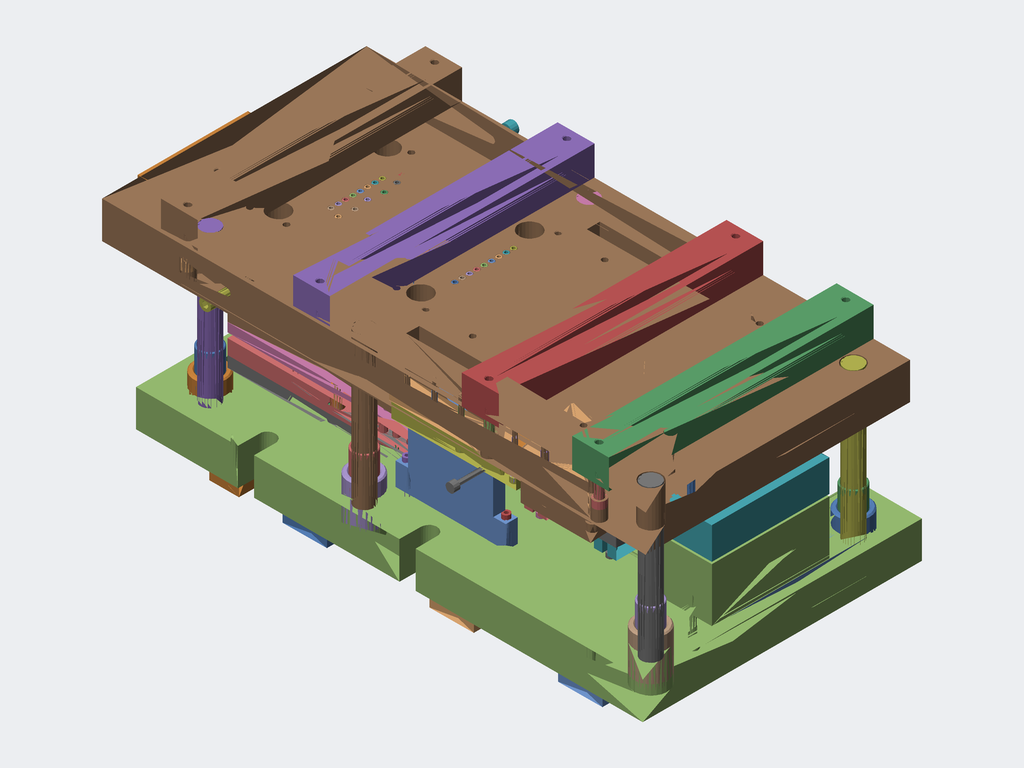Assembly | STEP file | 613 different items | 613 placed
Parts list (item | quantity | size | volume):
1 | x1 | 60 x 360 x 20 mm | 425296 mm3
2 | x1 | 40 x 360 x 20 mm | 281296 mm3
3 | x1 | 50 x 360 x 40 mm | 715429 mm3
4 | x1 | 50 x 360 x 40 mm | 715429 mm3
5 | x1 | 50 x 360 x 40 mm | 715429 mm3
6 | x1 | 50 x 360 x 40 mm | 715429 mm3
7 | x1 | 12 x 108 x 12 mm | 3732 mm3
8 | x1 | 12 x 108 x 12 mm | 3732 mm3
9 | x1 | 25 x 25 x 37 mm | 14578 mm3
10 | x1 | 6 x 42.771 x 14.853 mm | 2506 mm3
11 | x1 | 8 x 8 x 30 mm | 1498 mm3
12 | x1 | 8 x 8 x 30 mm | 1498 mm3
13 | x1 | 6 x 6 x 25 mm | 699.37 mm3
14 | x1 | 8 x 8 x 40 mm | 2000 mm3
15 | x1 | 8 x 8 x 40 mm | 2000 mm3
16 | x1 | 25 x 5 x 5 mm | 484.734 mm3
17 | x1 | 25 x 25 x 37 mm | 14578 mm3
18 | x1 | 24.97 x 5.97 x 55 mm | 8152 mm3
19 | x1 | 8 x 8 x 55 mm | 2684 mm3
20 | x1 | 8 x 8 x 30 mm | 1427 mm3
21 | x1 | 20 x 20 x 5 mm | 1265 mm3
22 | x1 | 6 x 6 x 36.5 mm | 342.826 mm3
23 | x1 | 6 x 6 x 36.5 mm | 342.826 mm3
24 | x1 | 6 x 6 x 36.5 mm | 342.826 mm3
25 | x1 | 6 x 6 x 36.5 mm | 342.826 mm3
26 | x1 | 6 x 6 x 36.5 mm | 342.826 mm3
27 | x1 | 6 x 6 x 36.5 mm | 342.826 mm3
28 | x1 | 6 x 6 x 36.5 mm | 342.826 mm3
29 | x1 | 6 x 6 x 36.5 mm | 342.826 mm3
30 | x1 | 6 x 6 x 36.5 mm | 342.826 mm3
31 | x1 | 6 x 6 x 36.5 mm | 342.826 mm3
32 | x1 | 6 x 6 x 36.5 mm | 342.826 mm3
33 | x1 | 6 x 6 x 36.5 mm | 342.826 mm3
34 | x1 | 6 x 6 x 36.5 mm | 342.826 mm3
35 | x1 | 6 x 6 x 36.5 mm | 342.826 mm3
36 | x1 | 6 x 6 x 36.5 mm | 342.826 mm3
37 | x1 | 6 x 6 x 36.5 mm | 342.826 mm3
38 | x1 | 6 x 6 x 36.5 mm | 342.826 mm3
39 | x1 | 6 x 6 x 36.5 mm | 342.826 mm3
40 | x1 | 6 x 6 x 36.5 mm | 342.826 mm3
41 | x1 | 6 x 6 x 36.5 mm | 342.826 mm3
42 | x1 | 6 x 6 x 36.5 mm | 342.826 mm3
43 | x1 | 6 x 6 x 36.5 mm | 342.826 mm3
44 | x1 | 6 x 6 x 36.5 mm | 342.826 mm3
45 | x1 | 6 x 6 x 36.5 mm | 342.826 mm3
46 | x1 | 5 x 5 x 25 mm | 484.734 mm3
47 | x1 | 12 x 12 x 4 mm | 331.627 mm3
48 | x1 | 12 x 12 x 4 mm | 331.627 mm3
49 | x1 | 12 x 12 x 4 mm | 331.627 mm3
50 | x1 | 12 x 12 x 4 mm | 331.627 mm3
51 | x1 | 12 x 12 x 4 mm | 331.627 mm3
52 | x1 | 12 x 12 x 4 mm | 331.627 mm3
53 | x1 | 8 x 8 x 50 mm | 2474 mm3
54 | x1 | 8 x 8 x 50 mm | 2474 mm3
55 | x1 | - | 125.363 mm3
56 | x1 | - | 125.363 mm3
57 | x1 | - | 125.363 mm3
58 | x1 | 29.97 x 5.97 x 55 mm | 9793 mm3
59 | x1 | 29.97 x 5.97 x 55 mm | 9793 mm3
60 | x1 | 24.97 x 9.97 x 55 mm | 13645 mm3
61 | x1 | 24.97 x 9.97 x 55 mm | 13645 mm3
62 | x1 | 25 x 130 x 15 mm | 47092 mm3
63 | x1 | 25 x 105.8 x 15 mm | 36908 mm3
64 | x1 | 25 x 16 x 80 mm | 27687 mm3
65 | x1 | 25 x 16 x 80 mm | 27687 mm3
66 | x1 | 150 x 150 x 43 mm | 782567 mm3
67 | x1 | 6 x 6 x 31.4 mm | 306.777 mm3
68 | x1 | 6 x 6 x 31.4 mm | 306.777 mm3
69 | x1 | 6 x 6 x 31.4 mm | 306.777 mm3
70 | x1 | 6 x 6 x 31.4 mm | 306.777 mm3
71 | x1 | 6 x 6 x 31.4 mm | 306.777 mm3
72 | x1 | 6 x 6 x 31.4 mm | 306.777 mm3
73 | x1 | 6 x 6 x 31.4 mm | 306.777 mm3
74 | x1 | 6 x 6 x 31.4 mm | 306.777 mm3
75 | x1 | 6 x 6 x 31.4 mm | 306.777 mm3
76 | x1 | 6 x 6 x 31.4 mm | 306.777 mm3
77 | x1 | 6 x 6 x 31.4 mm | 306.777 mm3
78 | x1 | 6 x 6 x 31.4 mm | 306.777 mm3
79 | x1 | 6 x 6 x 31.4 mm | 306.777 mm3
80 | x1 | 6 x 6 x 31.4 mm | 306.777 mm3
81 | x1 | 6 x 6 x 31.4 mm | 306.777 mm3
82 | x1 | 6 x 6 x 30.5 mm | 300.415 mm3
83 | x1 | 6 x 6 x 30.5 mm | 300.415 mm3
84 | x1 | 6 x 6 x 30.5 mm | 300.415 mm3
85 | x1 | 6 x 6 x 30.5 mm | 300.415 mm3
86 | x1 | 6 x 6 x 30.5 mm | 300.415 mm3
87 | x1 | 6 x 6 x 30.5 mm | 300.415 mm3
88 | x1 | 6 x 6 x 30.5 mm | 300.415 mm3
89 | x1 | 6 x 6 x 30.5 mm | 300.415 mm3
90 | x1 | 6 x 6 x 30.5 mm | 300.415 mm3
91 | x1 | 6 x 6 x 30.5 mm | 300.415 mm3
92 | x1 | 6 x 6 x 30.5 mm | 300.415 mm3
93 | x1 | 6 x 6 x 30.5 mm | 300.415 mm3
94 | x1 | 6 x 6 x 30.5 mm | 300.415 mm3
95 | x1 | 6 x 6 x 30.5 mm | 300.415 mm3
96 | x1 | 6 x 6 x 30.5 mm | 300.415 mm3
97 | x1 | 6 x 6 x 24.2 mm | 255.883 mm3
98 | x1 | 6 x 6 x 24.2 mm | 255.883 mm3
99 | x1 | 6 x 6 x 24.2 mm | 255.883 mm3
100 | x1 | 6 x 6 x 24.2 mm | 255.883 mm3
101 | x1 | 6 x 6 x 24.2 mm | 255.883 mm3
102 | x1 | 6 x 6 x 24.2 mm | 255.883 mm3
103 | x1 | 6 x 6 x 24.2 mm | 255.883 mm3
104 | x1 | 6 x 6 x 24.2 mm | 255.883 mm3
105 | x1 | 6 x 6 x 24.2 mm | 255.883 mm3
106 | x1 | 6 x 6 x 24.2 mm | 255.883 mm3
107 | x1 | 6 x 6 x 24.2 mm | 255.883 mm3
108 | x1 | 6 x 6 x 24.2 mm | 255.883 mm3
109 | x1 | 6 x 6 x 24.2 mm | 255.883 mm3
110 | x1 | 6 x 6 x 24.2 mm | 255.883 mm3
111 | x1 | 6 x 6 x 24.2 mm | 255.883 mm3
112 | x1 | 6 x 6 x 24.2 mm | 255.883 mm3
113 | x1 | 6 x 6 x 24.2 mm | 255.883 mm3
114 | x1 | 6 x 6 x 24.2 mm | 255.883 mm3
115 | x1 | 6 x 6 x 30.5 mm | 300.415 mm3
116 | x1 | 8 x 8 x 55 mm | 2726 mm3
117 | x1 | 8 x 8 x 55 mm | 2726 mm3
118 | x1 | 8 x 8 x 55 mm | 2726 mm3
119 | x1 | 8 x 8 x 55 mm | 2726 mm3
120 | x1 | 22 x 22 x 5 mm | 1608 mm3
121 | x1 | 170 x 20 x 20 mm | 54220 mm3
122 | x1 | 170 x 20 x 20 mm | 54220 mm3
123 | x1 | 275 x 320 x 12 mm | 986186 mm3
124 | x1 | 150 x 16 x 219.952 mm | 343529 mm3
125 | x1 | 114.24 x 2.3 x 30 mm | 5016 mm3
126 | x1 | 114.24 x 2.3 x 30 mm | 5016 mm3
127 | x1 | 114.24 x 2.3 x 30 mm | 5016 mm3
128 | x1 | 112 x 4.97 x 28.8 mm | 6489 mm3
129 | x1 | 112 x 4.97 x 28.8 mm | 6489 mm3
130 | x1 | 112 x 4.97 x 28.8 mm | 6489 mm3
131 | x1 | 110 x 5 x 24.6 mm | 7286 mm3
132 | x1 | 110 x 5 x 24.6 mm | 7286 mm3
133 | x1 | 110 x 5 x 24.6 mm | 7286 mm3
134 | x1 | 740 x 360 x 50 mm | 12464392 mm3
135 | x1 | 110 x 4.97 x 20 mm | 4432 mm3
136 | x1 | 110 x 4.97 x 20 mm | 4432 mm3
137 | x1 | 110 x 4.97 x 20 mm | 4432 mm3
138 | x1 | 110 x 4.97 x 20 mm | 4432 mm3
139 | x1 | 110 x 4.97 x 20 mm | 4432 mm3
140 | x1 | 114.24 x 2.3 x 30 mm | 5016 mm3
141 | x1 | 149 x 120 x 21.74 mm | 329380 mm3
142 | x1 | 28 x 28 x 35 mm | 8179 mm3
143 | x1 | 28 x 28 x 35 mm | 8179 mm3
144 | x1 | 28 x 28 x 35 mm | 8179 mm3
145 | x1 | 28 x 28 x 35 mm | 8179 mm3
146 | x1 | 28 x 28 x 35 mm | 8179 mm3
147 | x1 | 28 x 28 x 35 mm | 8179 mm3
148 | x1 | 28 x 28 x 35 mm | 8179 mm3
149 | x1 | 270 x 210 x 20 mm | 990769 mm3
150 | x1 | 270 x 210 x 20 mm | 665006 mm3
151 | x1 | 270 x 210 x 12 mm | 556019 mm3
152 | x1 | 270 x 210 x 15 mm | 687226 mm3
153 | x1 | 16 x 16 x 16 mm | 2762 mm3
154 | x1 | 22 x 17 x 50.8 mm | 13403 mm3
155 | x1 | 16 x 16 x 16 mm | 2762 mm3
156 | x1 | 22 x 100 x 29.5 mm | 60333 mm3
157 | x1 | 6 x 38.927 x 27.874 mm | 2506 mm3
158 | x1 | 30 x 210 x 15 mm | 89928 mm3
159 | x1 | 30 x 15 x 75 mm | 33035 mm3
160 | x1 | 22 x 17 x 50.8 mm | 13403 mm3
161 | x1 | 14 x 153 x 10 mm | 17764 mm3
162 | x1 | 60 x 288 x 31.2 mm | 374640 mm3
163 | x1 | 30 x 15 x 75 mm | 32986 mm3
164 | x1 | 27.92 x 20 x 22.9 mm | 8682 mm3
165 | x1 | 27.92 x 20 x 22.9 mm | 8682 mm3
166 | x1 | 95 x 320 x 31.2 mm | 758918 mm3
167 | x1 | 30 x 15 x 75 mm | 32980 mm3
168 | x1 | 30 x 15 x 75 mm | 33035 mm3
169 | x1 | 150 x 16 x 219.952 mm | 343529 mm3
170 | x1 | 30 x 210 x 15 mm | 89928 mm3
171 | x1 | 20 x 156 x 23.01 mm | 61919 mm3
172 | x1 | 22 x 17 x 50.8 mm | 13297 mm3
173 | x1 | 22 x 100 x 29.5 mm | 60684 mm3
174 | x1 | 14 x 153 x 10 mm | 17762 mm3
175 | x1 | 22 x 17 x 50.8 mm | 13297 mm3
176 | x1 | 110 x 5 x 24.6 mm | 7286 mm3
177 | x1 | 150 x 135 x 10 mm | 124052 mm3
178 | x1 | 118 x 5 x 53.54 mm | 21080 mm3
179 | x1 | 118 x 5 x 53.54 mm | 21081 mm3
180 | x1 | 118 x 5 x 53.54 mm | 21080 mm3
181 | x1 | 118 x 5 x 53.54 mm | 21081 mm3
182 | x1 | 118 x 5 x 53.54 mm | 21080 mm3
183 | x1 | 136 x 1.85 x 22 mm | 2666 mm3
184 | x1 | 136 x 1.85 x 22 mm | 2666 mm3
185 | x1 | 136 x 1.85 x 22 mm | 2666 mm3
186 | x1 | 136 x 1.85 x 22 mm | 2666 mm3
187 | x1 | 136 x 1.85 x 22 mm | 2666 mm3
188 | x1 | 136 x 1.85 x 22 mm | 2666 mm3
189 | x1 | 136 x 1.85 x 22 mm | 2666 mm3
190 | x1 | 136 x 1.85 x 22 mm | 2666 mm3
191 | x1 | 112 x 4.97 x 28.8 mm | 6489 mm3
192 | x1 | 28 x 28 x 35 mm | 8179 mm3
193 | x1 | 150 x 135 x 15 mm | 212258 mm3
194 | x1 | 39.94 x 2.4 x 27.2 mm | 2495 mm3
195 | x1 | 39.94 x 2.4 x 27.2 mm | 2495 mm3
196 | x1 | 39.94 x 2.4 x 27.2 mm | 2495 mm3
197 | x1 | 39.94 x 2.4 x 27.2 mm | 2495 mm3
198 | x1 | 39.94 x 2.4 x 27.2 mm | 2495 mm3
199 | x1 | 39.94 x 2.4 x 27.2 mm | 2495 mm3
200 | x1 | 39.94 x 2.4 x 27.2 mm | 2495 mm3
201 | x1 | 39.94 x 2.4 x 27.2 mm | 2495 mm3
202 | x1 | 39.94 x 2.4 x 27.2 mm | 2495 mm3
203 | x1 | 39.94 x 2.4 x 27.2 mm | 2495 mm3
204 | x1 | 39.94 x 2.4 x 27.2 mm | 2495 mm3
205 | x1 | 55 x 14 x 9.8 mm | 5918 mm3
206 | x1 | 60 x 14 x 9.8 mm | 6535 mm3
207 | x1 | 39.94 x 2.4 x 27.2 mm | 2495 mm3
208 | x1 | 39.94 x 2.4 x 27.2 mm | 2495 mm3
209 | x1 | 34.97 x 6 x 32.7 mm | 4654 mm3
210 | x1 | 34.97 x 6 x 32.7 mm | 4654 mm3
211 | x1 | 39.94 x 2.4 x 27.2 mm | 2495 mm3
212 | x1 | 39.94 x 2.4 x 27.2 mm | 2495 mm3
213 | x1 | 39.94 x 2.4 x 27.2 mm | 2495 mm3
214 | x1 | 39.94 x 2.4 x 27.2 mm | 2495 mm3
215 | x1 | 39.94 x 2.4 x 27.2 mm | 2495 mm3
216 | x1 | 22 x 22 x 5 mm | 1608 mm3
217 | x1 | 12 x 12 x 32 mm | 2552 mm3
218 | x1 | 12 x 12 x 32 mm | 2552 mm3
219 | x1 | 22 x 22 x 5 mm | 1608 mm3
220 | x1 | 22 x 22 x 5 mm | 1608 mm3
221 | x1 | 12 x 12 x 32 mm | 2552 mm3
222 | x1 | 22 x 22 x 5 mm | 1608 mm3
223 | x1 | 12 x 12 x 32 mm | 2552 mm3
224 | x1 | 22 x 22 x 5 mm | 1608 mm3
225 | x1 | 12 x 12 x 32 mm | 2552 mm3
226 | x1 | 16 x 16 x 27 mm | 3890 mm3
227 | x1 | 25 x 25 x 5 mm | 2168 mm3
228 | x1 | 16 x 16 x 27 mm | 3890 mm3
229 | x1 | 25 x 25 x 5 mm | 2168 mm3
230 | x1 | 16 x 16 x 27 mm | 3890 mm3
231 | x1 | 25 x 25 x 5 mm | 2168 mm3
232 | x1 | 25 x 25 x 5 mm | 2168 mm3
233 | x1 | 16 x 16 x 27 mm | 3890 mm3
234 | x1 | 16 x 16 x 27 mm | 3890 mm3
235 | x1 | 25 x 25 x 5 mm | 2168 mm3
236 | x1 | 16 x 16 x 27 mm | 3890 mm3
237 | x1 | 25 x 25 x 5 mm | 2168 mm3
238 | x1 | 16 x 16 x 27 mm | 3890 mm3
239 | x1 | 25 x 25 x 5 mm | 2168 mm3
240 | x1 | 14 x 14 x 27 mm | 2618 mm3
241 | x1 | 20 x 20 x 5 mm | 1265 mm3
242 | x1 | 14 x 14 x 27 mm | 2618 mm3
243 | x1 | 20 x 20 x 5 mm | 1265 mm3
244 | x1 | 14 x 14 x 27 mm | 2618 mm3
245 | x1 | 20 x 20 x 5 mm | 1265 mm3
246 | x1 | 14 x 14 x 27 mm | 2618 mm3
247 | x1 | 20 x 20 x 5 mm | 1265 mm3
248 | x1 | 14 x 14 x 27 mm | 2618 mm3
249 | x1 | 20 x 20 x 5 mm | 1265 mm3
250 | x1 | 25 x 25 x 5 mm | 2168 mm3
251 | x1 | 16 x 16 x 27 mm | 3890 mm3
252 | x1 | 14 x 14 x 27 mm | 2618 mm3
253 | x1 | 12 x 12 x 32 mm | 2552 mm3
254 | x1 | 270 x 210 x 20 mm | 936503 mm3
255 | x1 | 22 x 22 x 35 mm | 3894 mm3
256 | x1 | 22 x 22 x 35 mm | 3894 mm3
257 | x1 | 22 x 22 x 35 mm | 3894 mm3
258 | x1 | 22 x 22 x 35 mm | 3894 mm3
259 | x1 | 22 x 22 x 35 mm | 3894 mm3
260 | x1 | 22 x 22 x 35 mm | 3894 mm3
261 | x1 | 25 x 25 x 45 mm | 5947 mm3
262 | x1 | 25 x 25 x 45 mm | 5947 mm3
263 | x1 | 25 x 25 x 45 mm | 5947 mm3
264 | x1 | 25 x 25 x 45 mm | 5947 mm3
265 | x1 | 25 x 25 x 45 mm | 5947 mm3
266 | x1 | 25 x 25 x 45 mm | 5947 mm3
267 | x1 | 25 x 25 x 45 mm | 5947 mm3
268 | x1 | 25 x 25 x 45 mm | 5947 mm3
269 | x1 | 690 x 380 x 50 mm | 10135272 mm3
270 | x1 | 270 x 210 x 25 mm | 722658 mm3
271 | x1 | 12 x 12 x 46 mm | 1731 mm3
272 | x1 | 18 x 18 x 9.92 mm | 1371 mm3
273 | x1 | 20 x 156 x 23.01 mm | 61919 mm3
274 | x1 | 12 x 12 x 46 mm | 1731 mm3
275 | x1 | 18 x 18 x 9.92 mm | 1371 mm3
276 | x1 | 5.998 x 5.997 x 50.45 mm | 77.124 mm3
277 | x1 | 5.998 x 5.997 x 50.45 mm | 77.124 mm3
278 | x1 | 6 x 6 x 50 mm | 346.471 mm3
279 | x1 | 6 x 6 x 50 mm | 346.471 mm3
280 | x1 | 5.998 x 5.997 x 50.45 mm | 77.124 mm3
281 | x1 | 6 x 6 x 50 mm | 346.471 mm3
282 | x1 | 5.998 x 5.997 x 50.45 mm | 77.124 mm3
283 | x1 | 6 x 6 x 50 mm | 346.471 mm3
284 | x1 | 5.998 x 5.997 x 50.45 mm | 77.124 mm3
285 | x1 | 6 x 6 x 50 mm | 346.471 mm3
286 | x1 | 6 x 6 x 50 mm | 346.471 mm3
287 | x1 | 5.998 x 5.997 x 50.45 mm | 77.124 mm3
288 | x1 | 6 x 6 x 50 mm | 346.471 mm3
289 | x1 | 6 x 6 x 50 mm | 346.471 mm3
290 | x1 | 6 x 6 x 50 mm | 346.471 mm3
291 | x1 | 5.998 x 5.997 x 50.45 mm | 77.124 mm3
292 | x1 | 5.998 x 5.997 x 50.45 mm | 77.124 mm3
293 | x1 | 5.998 x 5.997 x 50.45 mm | 77.124 mm3
294 | x1 | 6 x 6 x 50 mm | 346.471 mm3
295 | x1 | 6 x 6 x 50 mm | 346.471 mm3
296 | x1 | 5.998 x 5.997 x 50.45 mm | 77.124 mm3
297 | x1 | 5.998 x 5.997 x 50.45 mm | 77.124 mm3
298 | x1 | 5.998 x 5.997 x 50.45 mm | 77.124 mm3
299 | x1 | 6 x 6 x 50 mm | 346.471 mm3
300 | x1 | 8 x 8 x 55 mm | 2684 mm3
301 | x1 | 8 x 8 x 55 mm | 2684 mm3
302 | x1 | 8 x 8 x 55 mm | 2684 mm3
303 | x1 | 8 x 8 x 30 mm | 1427 mm3
304 | x1 | 8 x 8 x 30 mm | 1427 mm3
305 | x1 | 8 x 8 x 30 mm | 1427 mm3
306 | x1 | 10 x 10 x 51 mm | 1658 mm3
307 | x1 | 10 x 10 x 51 mm | 1658 mm3
308 | x1 | 10 x 10 x 51 mm | 1658 mm3
309 | x1 | 10 x 10 x 51 mm | 1658 mm3
310 | x1 | 10 x 10 x 21 mm | 809.617 mm3
311 | x1 | 10 x 10 x 21 mm | 809.617 mm3
312 | x1 | 10 x 10 x 21 mm | 809.617 mm3
313 | x1 | 10 x 10 x 21 mm | 809.617 mm3
314 | x1 | 10 x 10 x 21 mm | 809.617 mm3
315 | x1 | 10 x 10 x 21 mm | 809.617 mm3
316 | x1 | 10 x 10 x 21 mm | 809.617 mm3
317 | x1 | 10 x 10 x 21 mm | 809.617 mm3
318 | x1 | 10 x 10 x 21 mm | 809.617 mm3
319 | x1 | 10 x 10 x 21 mm | 809.617 mm3
320 | x1 | 10 x 10 x 16 mm | 668.246 mm3
321 | x1 | 10 x 10 x 16 mm | 668.246 mm3
322 | x1 | 10 x 10 x 16 mm | 668.246 mm3
323 | x1 | 10 x 10 x 16 mm | 668.246 mm3
324 | x1 | 10 x 10 x 16 mm | 668.246 mm3
325 | x1 | 10 x 10 x 16 mm | 668.246 mm3
326 | x1 | 10 x 10 x 16 mm | 668.246 mm3
327 | x1 | 10 x 10 x 16 mm | 668.246 mm3
328 | x1 | 10 x 10 x 16 mm | 668.246 mm3
329 | x1 | 10 x 10 x 16 mm | 668.246 mm3
330 | x1 | 13 x 13 x 68 mm | 3913 mm3
331 | x1 | 13 x 13 x 68 mm | 3913 mm3
332 | x1 | 13 x 13 x 68 mm | 3913 mm3
333 | x1 | 13 x 13 x 68 mm | 3913 mm3
334 | x1 | 13 x 13 x 68 mm | 3913 mm3
335 | x1 | 13 x 13 x 68 mm | 3913 mm3
336 | x1 | 13 x 13 x 53 mm | 3159 mm3
337 | x1 | 13 x 13 x 53 mm | 3159 mm3
338 | x1 | 13 x 13 x 53 mm | 3159 mm3
339 | x1 | 13 x 13 x 53 mm | 3159 mm3
340 | x1 | 13 x 13 x 53 mm | 3159 mm3
341 | x1 | 13 x 13 x 53 mm | 3159 mm3
342 | x1 | 13 x 13 x 53 mm | 3159 mm3
343 | x1 | 13 x 13 x 53 mm | 3159 mm3
344 | x1 | 8 x 8 x 10 mm | 413.018 mm3
345 | x1 | 8 x 8 x 10 mm | 413.018 mm3
346 | x1 | 8 x 8 x 10 mm | 413.018 mm3
347 | x1 | 8 x 8 x 10 mm | 413.018 mm3
348 | x1 | 8 x 8 x 10 mm | 413.018 mm3
349 | x1 | 8 x 8 x 10 mm | 413.018 mm3
350 | x1 | 8 x 8 x 10 mm | 413.018 mm3
351 | x1 | 8 x 8 x 10 mm | 413.018 mm3
352 | x1 | 8 x 8 x 10 mm | 413.018 mm3
353 | x1 | 8 x 8 x 10 mm | 413.018 mm3
354 | x1 | 8 x 8 x 10 mm | 413.018 mm3
355 | x1 | 8 x 8 x 10 mm | 413.018 mm3
356 | x1 | 8 x 8 x 10 mm | 413.018 mm3
357 | x1 | 8 x 8 x 10 mm | 413.018 mm3
358 | x1 | 8 x 8 x 10 mm | 413.018 mm3
359 | x1 | 8 x 8 x 10 mm | 413.018 mm3
360 | x1 | 8 x 8 x 10 mm | 413.018 mm3
361 | x1 | 8 x 8 x 10 mm | 413.018 mm3
362 | x1 | 8 x 8 x 10 mm | 413.018 mm3
363 | x1 | 8 x 8 x 10 mm | 413.018 mm3
364 | x1 | 8 x 8 x 10 mm | 413.018 mm3
365 | x1 | 8 x 8 x 10 mm | 413.018 mm3
366 | x1 | 8 x 8 x 10 mm | 413.018 mm3
367 | x1 | 8 x 8 x 10 mm | 413.018 mm3
368 | x1 | 16 x 16 x 35 mm | 3608 mm3
369 | x1 | 16 x 16 x 35 mm | 3608 mm3
370 | x1 | 16 x 16 x 35 mm | 3608 mm3
371 | x1 | 16 x 16 x 35 mm | 3608 mm3
372 | x1 | 16 x 16 x 35 mm | 3608 mm3
373 | x1 | 16 x 16 x 35 mm | 3608 mm3
374 | x1 | 13 x 13 x 33 mm | 2154 mm3
375 | x1 | 13 x 13 x 33 mm | 2154 mm3
376 | x1 | 13 x 13 x 33 mm | 2154 mm3
377 | x1 | 13 x 13 x 33 mm | 2154 mm3
378 | x1 | 13 x 13 x 33 mm | 2154 mm3
379 | x1 | 13 x 13 x 33 mm | 2154 mm3
380 | x1 | 13 x 13 x 33 mm | 2154 mm3
381 | x1 | 13 x 13 x 33 mm | 2154 mm3
382 | x1 | 10 x 10 x 21 mm | 809.617 mm3
383 | x1 | 10 x 10 x 21 mm | 809.617 mm3
384 | x1 | 10 x 10 x 21 mm | 809.617 mm3
385 | x1 | 10 x 10 x 21 mm | 809.617 mm3
386 | x1 | 8.5 x 8.5 x 25 mm | 630.698 mm3
387 | x1 | 8.5 x 8.5 x 25 mm | 630.698 mm3
388 | x1 | 8.5 x 8.5 x 30 mm | 728.873 mm3
389 | x1 | 8.5 x 8.5 x 30 mm | 728.873 mm3
390 | x1 | 8.5 x 8.5 x 45 mm | 1023 mm3
391 | x1 | 8.5 x 8.5 x 45 mm | 1023 mm3
392 | x1 | 8.5 x 8.5 x 45 mm | 1023 mm3
393 | x1 | 16 x 50 x 16 mm | 4786 mm3
394 | x1 | 16 x 50 x 16 mm | 4786 mm3
395 | x1 | 16 x 16 x 50 mm | 4786 mm3
396 | x1 | 16 x 16 x 50 mm | 4786 mm3
397 | x1 | 16 x 16 x 50 mm | 4786 mm3
398 | x1 | 16 x 16 x 50 mm | 4786 mm3
399 | x1 | 16 x 16 x 50 mm | 4786 mm3
400 | x1 | 16 x 16 x 50 mm | 4786 mm3
401 | x1 | 16 x 16 x 50 mm | 4786 mm3
402 | x1 | 16 x 16 x 50 mm | 4786 mm3
403 | x1 | 13 x 13 x 58 mm | 3411 mm3
404 | x1 | 13 x 13 x 58 mm | 3411 mm3
405 | x1 | 13 x 13 x 58 mm | 3411 mm3
406 | x1 | 13 x 13 x 58 mm | 3411 mm3
407 | x1 | 13 x 13 x 58 mm | 3411 mm3
408 | x1 | 16 x 16 x 50 mm | 4786 mm3
409 | x1 | 16 x 16 x 50 mm | 4786 mm3
410 | x1 | 13 x 13 x 58 mm | 3411 mm3
411 | x1 | 10 x 10 x 21 mm | 809.617 mm3
412 | x1 | 10 x 10 x 21 mm | 809.617 mm3
413 | x1 | 10 x 10 x 21 mm | 809.617 mm3
414 | x1 | 10 x 10 x 21 mm | 809.617 mm3
415 | x1 | 10 x 10 x 21 mm | 809.617 mm3
416 | x1 | 10 x 10 x 21 mm | 809.617 mm3
417 | x1 | 13 x 13 x 48 mm | 2908 mm3
418 | x1 | 13 x 13 x 48 mm | 2908 mm3
419 | x1 | 5.5 x 5.5 x 48 mm | 378.644 mm3
420 | x1 | 5.5 x 5.5 x 48 mm | 378.644 mm3
421 | x1 | 5.5 x 5.5 x 48 mm | 378.644 mm3
422 | x1 | 5.5 x 5.5 x 48 mm | 378.644 mm3
423 | x1 | 5.5 x 5.5 x 48 mm | 378.644 mm3
424 | x1 | 5.5 x 5.5 x 48 mm | 378.644 mm3
425 | x1 | 5.5 x 5.5 x 48 mm | 378.644 mm3
426 | x1 | 5.5 x 5.5 x 48 mm | 378.644 mm3
427 | x1 | 8.5 x 8.5 x 25 mm | 577.553 mm3
428 | x1 | 8.5 x 8.5 x 25 mm | 577.553 mm3
429 | x1 | 8.5 x 8.5 x 25 mm | 577.553 mm3
430 | x1 | 8.5 x 8.5 x 25 mm | 577.553 mm3
431 | x1 | 10 x 10 x 21 mm | 809.617 mm3
432 | x1 | 10 x 10 x 21 mm | 809.617 mm3
433 | x1 | 10 x 10 x 21 mm | 809.617 mm3
434 | x1 | 10 x 10 x 21 mm | 809.617 mm3
435 | x1 | 10 x 10 x 21 mm | 809.617 mm3
436 | x1 | 10 x 10 x 21 mm | 809.617 mm3
437 | x1 | 10 x 10 x 21 mm | 809.617 mm3
438 | x1 | 10 x 10 x 21 mm | 809.617 mm3
439 | x1 | 10 x 10 x 36 mm | 1234 mm3
440 | x1 | 10 x 10 x 36 mm | 1234 mm3
441 | x1 | 10 x 10 x 36 mm | 1234 mm3
442 | x1 | 10 x 10 x 36 mm | 1234 mm3
443 | x1 | 10 x 10 x 51 mm | 1658 mm3
444 | x1 | 10 x 10 x 51 mm | 1658 mm3
445 | x1 | 10 x 10 x 51 mm | 1658 mm3
446 | x1 | 10 x 10 x 51 mm | 1658 mm3
447 | x1 | 10 x 10 x 51 mm | 1658 mm3
448 | x1 | 10 x 10 x 51 mm | 1658 mm3
449 | x1 | 10 x 10 x 51 mm | 1658 mm3
450 | x1 | 10 x 10 x 51 mm | 1658 mm3
451 | x1 | 10 x 10 x 51 mm | 1658 mm3
452 | x1 | 10 x 10 x 51 mm | 1658 mm3
453 | x1 | 13 x 13 x 58 mm | 3411 mm3
454 | x1 | 13 x 13 x 58 mm | 3411 mm3
455 | x1 | 13 x 13 x 58 mm | 3411 mm3
456 | x1 | 13 x 13 x 58 mm | 3411 mm3
457 | x1 | - | 70.891 mm3
458 | x1 | - | 70.891 mm3
459 | x1 | - | 70.891 mm3
460 | x1 | - | 70.891 mm3
461 | x1 | - | 70.891 mm3
462 | x1 | - | 70.891 mm3
463 | x1 | - | 70.891 mm3
464 | x1 | - | 70.891 mm3
465 | x1 | - | 70.891 mm3
466 | x1 | - | 70.891 mm3
467 | x1 | - | 70.891 mm3
468 | x1 | - | 70.891 mm3
469 | x1 | - | 70.891 mm3
470 | x1 | - | 70.891 mm3
471 | x1 | - | 70.891 mm3
472 | x1 | - | 70.891 mm3
473 | x1 | - | 70.891 mm3
474 | x1 | - | 70.891 mm3
475 | x1 | - | 70.891 mm3
476 | x1 | - | 70.891 mm3
477 | x1 | - | 70.891 mm3
478 | x1 | - | 70.891 mm3
479 | x1 | - | 70.891 mm3
480 | x1 | - | 70.891 mm3
481 | x1 | - | 70.891 mm3
482 | x1 | - | 70.891 mm3
483 | x1 | - | 70.891 mm3
484 | x1 | - | 70.891 mm3
485 | x1 | - | 70.891 mm3
486 | x1 | - | 70.891 mm3
487 | x1 | - | 70.891 mm3
488 | x1 | - | 70.891 mm3
489 | x1 | - | 70.891 mm3
490 | x1 | 6 x 6 x 40 mm | 281.648 mm3
491 | x1 | 6 x 6 x 40 mm | 281.648 mm3
492 | x1 | 6 x 6 x 40 mm | 281.648 mm3
493 | x1 | 6 x 6 x 40 mm | 281.648 mm3
494 | x1 | 6 x 6 x 40 mm | 281.648 mm3
495 | x1 | 6 x 6 x 40 mm | 281.648 mm3
496 | x1 | 6 x 6 x 40 mm | 281.648 mm3
497 | x1 | 6 x 6 x 40 mm | 281.648 mm3
498 | x1 | 6 x 6 x 40 mm | 281.648 mm3
499 | x1 | 6 x 6 x 40 mm | 281.648 mm3
500 | x1 | 6 x 6 x 40 mm | 281.648 mm3
501 | x1 | 6 x 6 x 40 mm | 281.648 mm3
502 | x1 | 6 x 6 x 40 mm | 281.648 mm3
503 | x1 | 6 x 6 x 40 mm | 281.648 mm3
504 | x1 | - | 70.891 mm3
505 | x1 | 6 x 6 x 40 mm | 281.648 mm3
506 | x1 | 8 x 8 x 10 mm | 413.018 mm3
507 | x1 | 8 x 8 x 10 mm | 413.018 mm3
508 | x1 | 8 x 8 x 10 mm | 413.018 mm3
509 | x1 | 8 x 8 x 10 mm | 413.018 mm3
510 | x1 | 8 x 8 x 10 mm | 413.018 mm3
511 | x1 | 8 x 8 x 10 mm | 413.018 mm3
512 | x1 | 8 x 8 x 10 mm | 413.018 mm3
513 | x1 | 8 x 8 x 10 mm | 413.018 mm3
514 | x1 | 8 x 8 x 10 mm | 413.018 mm3
515 | x1 | 8 x 8 x 10 mm | 413.018 mm3
516 | x1 | 8 x 8 x 10 mm | 413.018 mm3
517 | x1 | 8 x 8 x 10 mm | 413.018 mm3
518 | x1 | 8 x 8 x 10 mm | 413.018 mm3
519 | x1 | 8 x 8 x 10 mm | 413.018 mm3
520 | x1 | 8 x 8 x 10 mm | 413.018 mm3
521 | x1 | 8 x 8 x 10 mm | 413.018 mm3
522 | x1 | 8 x 8 x 10 mm | 413.018 mm3
523 | x1 | 8 x 8 x 10 mm | 413.018 mm3
524 | x1 | 8 x 8 x 10 mm | 413.018 mm3
525 | x1 | 8 x 8 x 10 mm | 413.018 mm3
526 | x1 | 8 x 8 x 10 mm | 413.018 mm3
527 | x1 | 8 x 8 x 10 mm | 413.018 mm3
528 | x1 | 8 x 8 x 10 mm | 413.018 mm3
529 | x1 | 8 x 8 x 10 mm | 413.018 mm3
530 | x1 | 8 x 8 x 10 mm | 413.018 mm3
531 | x1 | 8 x 8 x 10 mm | 413.018 mm3
532 | x1 | 8 x 8 x 10 mm | 413.018 mm3
533 | x1 | 8 x 8 x 10 mm | 413.018 mm3
534 | x1 | 8 x 8 x 10 mm | 413.018 mm3
535 | x1 | 8 x 8 x 10 mm | 413.018 mm3
536 | x1 | 8 x 8 x 10 mm | 413.018 mm3
537 | x1 | 8 x 8 x 10 mm | 413.018 mm3
538 | x1 | 8 x 8 x 10 mm | 413.018 mm3
539 | x1 | 8 x 8 x 10 mm | 413.018 mm3
540 | x1 | 8 x 8 x 10 mm | 413.018 mm3
541 | x1 | 8 x 8 x 10 mm | 413.018 mm3
542 | x1 | 8 x 8 x 10 mm | 413.018 mm3
543 | x1 | 8 x 8 x 10 mm | 413.018 mm3
544 | x1 | 8 x 8 x 10 mm | 413.018 mm3
545 | x1 | 8 x 8 x 10 mm | 413.018 mm3
546 | x1 | 8 x 8 x 10 mm | 413.018 mm3
547 | x1 | 8 x 8 x 10 mm | 413.018 mm3
548 | x1 | 8 x 8 x 10 mm | 413.018 mm3
549 | x1 | 8 x 8 x 10 mm | 413.018 mm3
550 | x1 | 8 x 8 x 10 mm | 413.018 mm3
551 | x1 | 8 x 8 x 10 mm | 413.018 mm3
552 | x1 | 8 x 8 x 10 mm | 413.018 mm3
553 | x1 | 8 x 8 x 10 mm | 413.018 mm3
554 | x1 | 8 x 8 x 10 mm | 413.018 mm3
555 | x1 | 5 x 5 x 25 mm | 484.734 mm3
556 | x1 | 5 x 5 x 25 mm | 484.734 mm3
557 | x1 | 5 x 5 x 25 mm | 484.734 mm3
558 | x1 | 31 x 31 x 60 mm | 12837 mm3
559 | x1 | 44 x 44 x 70 mm | 53175 mm3
560 | x1 | 29 x 29 x 10 mm | 913.883 mm3
561 | x1 | 31 x 31 x 60 mm | 12837 mm3
562 | x1 | 44 x 44 x 70 mm | 53175 mm3
563 | x1 | 29 x 29 x 10 mm | 913.883 mm3
564 | x1 | 44 x 44 x 70 mm | 53175 mm3
565 | x1 | 31 x 31 x 60 mm | 12837 mm3
566 | x1 | 29 x 29 x 10 mm | 913.883 mm3
567 | x1 | 29 x 29 x 10 mm | 913.883 mm3
568 | x1 | 31 x 31 x 60 mm | 12837 mm3
569 | x1 | 44 x 44 x 70 mm | 53175 mm3
570 | x1 | 6 x 38.927 x 27.874 mm | 2506 mm3
571 | x1 | 25 x 5 x 5 mm | 484.734 mm3
572 | x1 | 25 x 5 x 5 mm | 484.734 mm3
573 | x1 | 25 x 5 x 5 mm | 484.734 mm3
574 | x1 | 25 x 5 x 5 mm | 484.734 mm3
575 | x1 | 94 x 8 x 8 mm | 1968 mm3
576 | x1 | 94 x 8 x 8 mm | 1968 mm3
577 | x1 | 94 x 8 x 8 mm | 1968 mm3
578 | x1 | 94 x 8 x 8 mm | 1968 mm3
579 | x1 | 6 x 42.771 x 14.853 mm | 2506 mm3
580 | x1 | 25 x 5 x 5 mm | 484.734 mm3
581 | x1 | 25 x 5 x 5 mm | 484.734 mm3
582 | x1 | 25 x 5 x 5 mm | 484.734 mm3
583 | x1 | 6 x 6 x 25 mm | 699.37 mm3
584 | x1 | 6 x 6 x 25 mm | 699.37 mm3
585 | x1 | 6 x 6 x 25 mm | 699.37 mm3
586 | x1 | 80 x 160 x 43.2 mm | 550360 mm3
587 | x1 | 60 x 360 x 20 mm | 425296 mm3
588 | x1 | 60 x 360 x 20 mm | 425296 mm3
589 | x1 | 80 x 160 x 72.8 mm | 929967 mm3
590 | x1 | 29 x 29 x 10 mm | 913.883 mm3
591 | x1 | 31 x 31 x 60 mm | 12837 mm3
592 | x1 | 44 x 44 x 70 mm | 53175 mm3
593 | x1 | 44 x 44 x 70 mm | 53175 mm3
594 | x1 | 29 x 29 x 10 mm | 913.883 mm3
595 | x1 | 31 x 31 x 60 mm | 12837 mm3
596 | x1 | 25 x 25 x 210 mm | 102898 mm3
597 | x1 | 25 x 25 x 210 mm | 102898 mm3
598 | x1 | 25 x 25 x 210 mm | 102898 mm3
599 | x1 | 25 x 25 x 210 mm | 102898 mm3
600 | x1 | 25 x 25 x 210 mm | 102898 mm3
601 | x1 | 25 x 25 x 210 mm | 102898 mm3
602 | x1 | 20 x 20 x 16 mm | 3516 mm3
603 | x1 | 20 x 20 x 16 mm | 3516 mm3
604 | x1 | 20 x 20 x 16 mm | 3516 mm3
605 | x1 | 20 x 20 x 16 mm | 3516 mm3
606 | x1 | 23 x 23 x 110 mm | 23077 mm3
607 | x1 | 23 x 23 x 110 mm | 23077 mm3
608 | x1 | 23 x 23 x 110 mm | 23077 mm3
609 | x1 | 23 x 23 x 110 mm | 23077 mm3
610 | x1 | 20 x 20 x 16 mm | 3516 mm3
611 | x1 | 20 x 20 x 16 mm | 3516 mm3
612 | x1 | 20 x 20 x 16 mm | 3516 mm3
613 | x1 | 20 x 20 x 16 mm | 3516 mm3
Placements (level | parent | child | x y z in mm | rotation matrix by rows), first 233 of 613 lines:
1 | subassembly 2 | subassembly 3 | 0.0 0.0 0.0 | 1 0 0 0 1 0 0 0 1
1 | subassembly 2 | subassembly 4 | 0.0 0.0 0.0 | 1 0 0 0 1 0 0 0 1
1 | subassembly 2 | subassembly 5 | 0.0 0.0 0.0 | 1 0 0 0 1 0 0 0 1
1 | subassembly 2 | subassembly 6 | 0.0 0.0 0.0 | 1 0 0 0 1 0 0 0 1
1 | subassembly 2 | subassembly 7 | 0.0 0.0 0.0 | 1 0 0 0 1 0 0 0 1
1 | subassembly 2 | subassembly 8 | 0.0 0.0 0.0 | 1 0 0 0 1 0 0 0 1
1 | subassembly 2 | subassembly 9 | 0.0 0.0 0.0 | 1 0 0 0 1 0 0 0 1
1 | subassembly 2 | subassembly 10 | 0.0 0.0 0.0 | 1 0 0 0 1 0 0 0 1
1 | subassembly 2 | subassembly 11 | 0.0 0.0 0.0 | 1 0 0 0 1 0 0 0 1
1 | subassembly 2 | subassembly 12 | 0.0 0.0 0.0 | 1 0 0 0 1 0 0 0 1
1 | subassembly 2 | subassembly 13 | 0.0 0.0 0.0 | 1 0 0 0 1 0 0 0 1
1 | subassembly 2 | subassembly 14 | 0.0 0.0 0.0 | 1 0 0 0 1 0 0 0 1
1 | subassembly 2 | subassembly 15 | 0.0 0.0 0.0 | 1 0 0 0 1 0 0 0 1
1 | subassembly 2 | subassembly 16 | 0.0 0.0 0.0 | 1 0 0 0 1 0 0 0 1
1 | subassembly 2 | subassembly 17 | 0.0 0.0 0.0 | 1 0 0 0 1 0 0 0 1
1 | subassembly 2 | subassembly 18 | 0.0 0.0 0.0 | 1 0 0 0 1 0 0 0 1
1 | subassembly 2 | subassembly 19 | 0.0 0.0 0.0 | 1 0 0 0 1 0 0 0 1
1 | subassembly 2 | subassembly 20 | 0.0 0.0 0.0 | 1 0 0 0 1 0 0 0 1
1 | subassembly 2 | subassembly 21 | 0.0 0.0 0.0 | 1 0 0 0 1 0 0 0 1
1 | subassembly 2 | subassembly 22 | 0.0 0.0 0.0 | 1 0 0 0 1 0 0 0 1
1 | subassembly 2 | subassembly 23 | 0.0 0.0 0.0 | 1 0 0 0 1 0 0 0 1
1 | subassembly 2 | subassembly 24 | 0.0 0.0 0.0 | 1 0 0 0 1 0 0 0 1
1 | subassembly 2 | subassembly 25 | 0.0 0.0 0.0 | 1 0 0 0 1 0 0 0 1
1 | subassembly 2 | subassembly 26 | 0.0 0.0 0.0 | 1 0 0 0 1 0 0 0 1
1 | subassembly 2 | subassembly 27 | 0.0 0.0 0.0 | 1 0 0 0 1 0 0 0 1
1 | subassembly 2 | subassembly 28 | 0.0 0.0 0.0 | 1 0 0 0 1 0 0 0 1
1 | subassembly 2 | subassembly 29 | 0.0 0.0 0.0 | 1 0 0 0 1 0 0 0 1
1 | subassembly 2 | subassembly 30 | 0.0 0.0 0.0 | 1 0 0 0 1 0 0 0 1
1 | subassembly 2 | subassembly 31 | 0.0 0.0 0.0 | 1 0 0 0 1 0 0 0 1
1 | subassembly 2 | subassembly 32 | 0.0 0.0 0.0 | 1 0 0 0 1 0 0 0 1
1 | subassembly 2 | subassembly 33 | 0.0 0.0 0.0 | 1 0 0 0 1 0 0 0 1
1 | subassembly 2 | subassembly 34 | 0.0 0.0 0.0 | 1 0 0 0 1 0 0 0 1
1 | subassembly 2 | subassembly 35 | 0.0 0.0 0.0 | 1 0 0 0 1 0 0 0 1
1 | subassembly 2 | subassembly 36 | 0.0 0.0 0.0 | 1 0 0 0 1 0 0 0 1
1 | subassembly 2 | subassembly 37 | 0.0 0.0 0.0 | 1 0 0 0 1 0 0 0 1
1 | subassembly 2 | subassembly 38 | 0.0 0.0 0.0 | 1 0 0 0 1 0 0 0 1
1 | subassembly 2 | subassembly 39 | 0.0 0.0 0.0 | 1 0 0 0 1 0 0 0 1
1 | subassembly 2 | subassembly 40 | 0.0 0.0 0.0 | 1 0 0 0 1 0 0 0 1
1 | subassembly 2 | subassembly 41 | 0.0 0.0 0.0 | 1 0 0 0 1 0 0 0 1
1 | subassembly 2 | subassembly 42 | 0.0 0.0 0.0 | 1 0 0 0 1 0 0 0 1
1 | subassembly 2 | subassembly 43 | 0.0 0.0 0.0 | 1 0 0 0 1 0 0 0 1
1 | subassembly 2 | subassembly 44 | 0.0 0.0 0.0 | 1 0 0 0 1 0 0 0 1
1 | subassembly 2 | subassembly 45 | 0.0 0.0 0.0 | 1 0 0 0 1 0 0 0 1
1 | subassembly 2 | subassembly 46 | 0.0 0.0 0.0 | 1 0 0 0 1 0 0 0 1
1 | subassembly 2 | subassembly 47 | 0.0 0.0 0.0 | 1 0 0 0 1 0 0 0 1
1 | subassembly 2 | subassembly 48 | 0.0 0.0 0.0 | 1 0 0 0 1 0 0 0 1
1 | subassembly 2 | subassembly 49 | 0.0 0.0 0.0 | 1 0 0 0 1 0 0 0 1
1 | subassembly 2 | subassembly 50 | 0.0 0.0 0.0 | 1 0 0 0 1 0 0 0 1
1 | subassembly 2 | subassembly 51 | 0.0 0.0 0.0 | 1 0 0 0 1 0 0 0 1
1 | subassembly 2 | subassembly 52 | 0.0 0.0 0.0 | 1 0 0 0 1 0 0 0 1
1 | subassembly 2 | subassembly 53 | 0.0 0.0 0.0 | 1 0 0 0 1 0 0 0 1
1 | subassembly 2 | subassembly 54 | 0.0 0.0 0.0 | 1 0 0 0 1 0 0 0 1
1 | subassembly 2 | subassembly 55 | 0.0 0.0 0.0 | 1 0 0 0 1 0 0 0 1
1 | subassembly 2 | subassembly 56 | 0.0 0.0 0.0 | 1 0 0 0 1 0 0 0 1
1 | subassembly 2 | subassembly 57 | 0.0 0.0 0.0 | 1 0 0 0 1 0 0 0 1
1 | subassembly 2 | subassembly 58 | 0.0 0.0 0.0 | 1 0 0 0 1 0 0 0 1
1 | subassembly 2 | subassembly 59 | 0.0 0.0 0.0 | 1 0 0 0 1 0 0 0 1
1 | subassembly 2 | subassembly 60 | 0.0 0.0 0.0 | 1 0 0 0 1 0 0 0 1
1 | subassembly 2 | subassembly 61 | 0.0 0.0 0.0 | 1 0 0 0 1 0 0 0 1
1 | subassembly 2 | subassembly 62 | 0.0 0.0 0.0 | 1 0 0 0 1 0 0 0 1
1 | subassembly 2 | subassembly 63 | 0.0 0.0 0.0 | 1 0 0 0 1 0 0 0 1
1 | subassembly 2 | subassembly 64 | 0.0 0.0 0.0 | 1 0 0 0 1 0 0 0 1
1 | subassembly 2 | subassembly 65 | 0.0 0.0 0.0 | 1 0 0 0 1 0 0 0 1
1 | subassembly 2 | subassembly 66 | 0.0 0.0 0.0 | 1 0 0 0 1 0 0 0 1
1 | subassembly 2 | subassembly 67 | 0.0 0.0 0.0 | 1 0 0 0 1 0 0 0 1
1 | subassembly 2 | subassembly 68 | 0.0 0.0 0.0 | 1 0 0 0 1 0 0 0 1
1 | subassembly 2 | subassembly 69 | 0.0 0.0 0.0 | 1 0 0 0 1 0 0 0 1
1 | subassembly 2 | subassembly 70 | 0.0 0.0 0.0 | 1 0 0 0 1 0 0 0 1
1 | subassembly 2 | subassembly 71 | 0.0 0.0 0.0 | 1 0 0 0 1 0 0 0 1
1 | subassembly 2 | subassembly 72 | 0.0 0.0 0.0 | 1 0 0 0 1 0 0 0 1
1 | subassembly 2 | subassembly 73 | 0.0 0.0 0.0 | 1 0 0 0 1 0 0 0 1
1 | subassembly 2 | subassembly 74 | 0.0 0.0 0.0 | 1 0 0 0 1 0 0 0 1
1 | subassembly 2 | subassembly 75 | 0.0 0.0 0.0 | 1 0 0 0 1 0 0 0 1
1 | subassembly 2 | subassembly 76 | 0.0 0.0 0.0 | 1 0 0 0 1 0 0 0 1
1 | subassembly 2 | subassembly 77 | 0.0 0.0 0.0 | 1 0 0 0 1 0 0 0 1
1 | subassembly 2 | subassembly 78 | 0.0 0.0 0.0 | 1 0 0 0 1 0 0 0 1
1 | subassembly 2 | subassembly 79 | 0.0 0.0 0.0 | 1 0 0 0 1 0 0 0 1
1 | subassembly 2 | subassembly 80 | 0.0 0.0 0.0 | 1 0 0 0 1 0 0 0 1
1 | subassembly 2 | subassembly 81 | 0.0 0.0 0.0 | 1 0 0 0 1 0 0 0 1
1 | subassembly 2 | subassembly 82 | 0.0 0.0 0.0 | 1 0 0 0 1 0 0 0 1
1 | subassembly 2 | subassembly 83 | 0.0 0.0 0.0 | 1 0 0 0 1 0 0 0 1
1 | subassembly 2 | subassembly 84 | 0.0 0.0 0.0 | 1 0 0 0 1 0 0 0 1
1 | subassembly 2 | subassembly 85 | 0.0 0.0 0.0 | 1 0 0 0 1 0 0 0 1
1 | subassembly 2 | subassembly 86 | 0.0 0.0 0.0 | 1 0 0 0 1 0 0 0 1
1 | subassembly 2 | subassembly 87 | 0.0 0.0 0.0 | 1 0 0 0 1 0 0 0 1
1 | subassembly 2 | subassembly 88 | 0.0 0.0 0.0 | 1 0 0 0 1 0 0 0 1
1 | subassembly 2 | subassembly 89 | 0.0 0.0 0.0 | 1 0 0 0 1 0 0 0 1
1 | subassembly 2 | subassembly 90 | 0.0 0.0 0.0 | 1 0 0 0 1 0 0 0 1
1 | subassembly 2 | subassembly 91 | 0.0 0.0 0.0 | 1 0 0 0 1 0 0 0 1
1 | subassembly 2 | subassembly 92 | 0.0 0.0 0.0 | 1 0 0 0 1 0 0 0 1
1 | subassembly 2 | subassembly 93 | 0.0 0.0 0.0 | 1 0 0 0 1 0 0 0 1
1 | subassembly 2 | subassembly 94 | 0.0 0.0 0.0 | 1 0 0 0 1 0 0 0 1
1 | subassembly 2 | subassembly 95 | 0.0 0.0 0.0 | 1 0 0 0 1 0 0 0 1
1 | subassembly 2 | subassembly 96 | 0.0 0.0 0.0 | 1 0 0 0 1 0 0 0 1
1 | subassembly 2 | subassembly 97 | 0.0 0.0 0.0 | 1 0 0 0 1 0 0 0 1
1 | subassembly 2 | subassembly 98 | 0.0 0.0 0.0 | 1 0 0 0 1 0 0 0 1
1 | subassembly 2 | subassembly 99 | 0.0 0.0 0.0 | 1 0 0 0 1 0 0 0 1
1 | subassembly 2 | subassembly 100 | 0.0 0.0 0.0 | 1 0 0 0 1 0 0 0 1
1 | subassembly 2 | subassembly 101 | 0.0 0.0 0.0 | 1 0 0 0 1 0 0 0 1
1 | subassembly 2 | subassembly 102 | 0.0 0.0 0.0 | 1 0 0 0 1 0 0 0 1
1 | subassembly 2 | subassembly 103 | 0.0 0.0 0.0 | 1 0 0 0 1 0 0 0 1
1 | subassembly 2 | subassembly 104 | 0.0 0.0 0.0 | 1 0 0 0 1 0 0 0 1
1 | subassembly 2 | subassembly 105 | 0.0 0.0 0.0 | 1 0 0 0 1 0 0 0 1
1 | subassembly 2 | subassembly 106 | 0.0 0.0 0.0 | 1 0 0 0 1 0 0 0 1
1 | subassembly 2 | subassembly 107 | 0.0 0.0 0.0 | 1 0 0 0 1 0 0 0 1
1 | subassembly 2 | subassembly 108 | 0.0 0.0 0.0 | 1 0 0 0 1 0 0 0 1
1 | subassembly 2 | subassembly 109 | 0.0 0.0 0.0 | 1 0 0 0 1 0 0 0 1
1 | subassembly 2 | subassembly 110 | 0.0 0.0 0.0 | 1 0 0 0 1 0 0 0 1
1 | subassembly 2 | subassembly 111 | 0.0 0.0 0.0 | 1 0 0 0 1 0 0 0 1
1 | subassembly 2 | subassembly 112 | 0.0 0.0 0.0 | 1 0 0 0 1 0 0 0 1
1 | subassembly 2 | subassembly 113 | 0.0 0.0 0.0 | 1 0 0 0 1 0 0 0 1
1 | subassembly 2 | subassembly 114 | 0.0 0.0 0.0 | 1 0 0 0 1 0 0 0 1
1 | subassembly 2 | subassembly 115 | 0.0 0.0 0.0 | 1 0 0 0 1 0 0 0 1
1 | subassembly 2 | subassembly 116 | 0.0 0.0 0.0 | 1 0 0 0 1 0 0 0 1
1 | subassembly 2 | subassembly 117 | 0.0 0.0 0.0 | 1 0 0 0 1 0 0 0 1
1 | subassembly 2 | subassembly 118 | 0.0 0.0 0.0 | 1 0 0 0 1 0 0 0 1
1 | subassembly 2 | subassembly 119 | 0.0 0.0 0.0 | 1 0 0 0 1 0 0 0 1
1 | subassembly 2 | subassembly 120 | 0.0 0.0 0.0 | 1 0 0 0 1 0 0 0 1
1 | subassembly 2 | subassembly 121 | 0.0 0.0 0.0 | 1 0 0 0 1 0 0 0 1
1 | subassembly 2 | subassembly 122 | 0.0 0.0 0.0 | 1 0 0 0 1 0 0 0 1
1 | subassembly 2 | subassembly 123 | 0.0 0.0 0.0 | 1 0 0 0 1 0 0 0 1
1 | subassembly 2 | subassembly 124 | 0.0 0.0 0.0 | 1 0 0 0 1 0 0 0 1
1 | subassembly 2 | subassembly 125 | 0.0 0.0 0.0 | 1 0 0 0 1 0 0 0 1
1 | subassembly 2 | subassembly 126 | 0.0 0.0 0.0 | 1 0 0 0 1 0 0 0 1
1 | subassembly 2 | subassembly 127 | 0.0 0.0 0.0 | 1 0 0 0 1 0 0 0 1
1 | subassembly 2 | subassembly 128 | 0.0 0.0 0.0 | 1 0 0 0 1 0 0 0 1
1 | subassembly 2 | subassembly 129 | 0.0 0.0 0.0 | 1 0 0 0 1 0 0 0 1
1 | subassembly 2 | subassembly 130 | 0.0 0.0 0.0 | 1 0 0 0 1 0 0 0 1
1 | subassembly 2 | subassembly 131 | 0.0 0.0 0.0 | 1 0 0 0 1 0 0 0 1
1 | subassembly 2 | subassembly 132 | 0.0 0.0 0.0 | 1 0 0 0 1 0 0 0 1
1 | subassembly 2 | subassembly 133 | 0.0 0.0 0.0 | 1 0 0 0 1 0 0 0 1
1 | subassembly 2 | subassembly 134 | 0.0 0.0 0.0 | 1 0 0 0 1 0 0 0 1
1 | subassembly 2 | subassembly 135 | 0.0 0.0 0.0 | 1 0 0 0 1 0 0 0 1
1 | subassembly 2 | subassembly 136 | 0.0 0.0 0.0 | 1 0 0 0 1 0 0 0 1
1 | subassembly 2 | subassembly 137 | 0.0 0.0 0.0 | 1 0 0 0 1 0 0 0 1
1 | subassembly 2 | subassembly 138 | 0.0 0.0 0.0 | 1 0 0 0 1 0 0 0 1
1 | subassembly 2 | subassembly 139 | 0.0 0.0 0.0 | 1 0 0 0 1 0 0 0 1
1 | subassembly 2 | subassembly 140 | 0.0 0.0 0.0 | 1 0 0 0 1 0 0 0 1
1 | subassembly 2 | subassembly 141 | 0.0 0.0 0.0 | 1 0 0 0 1 0 0 0 1
1 | subassembly 2 | subassembly 142 | 0.0 0.0 0.0 | 1 0 0 0 1 0 0 0 1
1 | subassembly 2 | subassembly 143 | 0.0 0.0 0.0 | 1 0 0 0 1 0 0 0 1
1 | subassembly 2 | subassembly 144 | 0.0 0.0 0.0 | 1 0 0 0 1 0 0 0 1
1 | subassembly 2 | subassembly 145 | 0.0 0.0 0.0 | 1 0 0 0 1 0 0 0 1
1 | subassembly 2 | subassembly 146 | 0.0 0.0 0.0 | 1 0 0 0 1 0 0 0 1
1 | subassembly 2 | subassembly 147 | 0.0 0.0 0.0 | 1 0 0 0 1 0 0 0 1
1 | subassembly 2 | subassembly 148 | 0.0 0.0 0.0 | 1 0 0 0 1 0 0 0 1
1 | subassembly 2 | subassembly 149 | 0.0 0.0 0.0 | 1 0 0 0 1 0 0 0 1
1 | subassembly 2 | subassembly 150 | 0.0 0.0 0.0 | 1 0 0 0 1 0 0 0 1
1 | subassembly 2 | subassembly 151 | 0.0 0.0 0.0 | 1 0 0 0 1 0 0 0 1
1 | subassembly 2 | subassembly 152 | 0.0 0.0 0.0 | 1 0 0 0 1 0 0 0 1
1 | subassembly 2 | subassembly 153 | 0.0 0.0 0.0 | 1 0 0 0 1 0 0 0 1
1 | subassembly 2 | subassembly 154 | 0.0 0.0 0.0 | 1 0 0 0 1 0 0 0 1
1 | subassembly 2 | subassembly 155 | 0.0 0.0 0.0 | 1 0 0 0 1 0 0 0 1
1 | subassembly 2 | subassembly 156 | 0.0 0.0 0.0 | 1 0 0 0 1 0 0 0 1
1 | subassembly 2 | subassembly 157 | 0.0 0.0 0.0 | 1 0 0 0 1 0 0 0 1
1 | subassembly 2 | subassembly 158 | 0.0 0.0 0.0 | 1 0 0 0 1 0 0 0 1
1 | subassembly 2 | subassembly 159 | 0.0 0.0 0.0 | 1 0 0 0 1 0 0 0 1
1 | subassembly 2 | subassembly 160 | 0.0 0.0 0.0 | 1 0 0 0 1 0 0 0 1
1 | subassembly 2 | subassembly 161 | 0.0 0.0 0.0 | 1 0 0 0 1 0 0 0 1
1 | subassembly 2 | subassembly 162 | 0.0 0.0 0.0 | 1 0 0 0 1 0 0 0 1
1 | subassembly 2 | subassembly 163 | 0.0 0.0 0.0 | 1 0 0 0 1 0 0 0 1
1 | subassembly 2 | subassembly 164 | 0.0 0.0 0.0 | 1 0 0 0 1 0 0 0 1
1 | subassembly 2 | subassembly 165 | 0.0 0.0 0.0 | 1 0 0 0 1 0 0 0 1
1 | subassembly 2 | subassembly 166 | 0.0 0.0 0.0 | 1 0 0 0 1 0 0 0 1
1 | subassembly 2 | subassembly 167 | 0.0 0.0 0.0 | 1 0 0 0 1 0 0 0 1
1 | subassembly 2 | subassembly 168 | 0.0 0.0 0.0 | 1 0 0 0 1 0 0 0 1
1 | subassembly 2 | subassembly 169 | 0.0 0.0 0.0 | 1 0 0 0 1 0 0 0 1
1 | subassembly 2 | subassembly 170 | 0.0 0.0 0.0 | 1 0 0 0 1 0 0 0 1
1 | subassembly 2 | subassembly 171 | 0.0 0.0 0.0 | 1 0 0 0 1 0 0 0 1
1 | subassembly 2 | subassembly 172 | 0.0 0.0 0.0 | 1 0 0 0 1 0 0 0 1
1 | subassembly 2 | subassembly 173 | 0.0 0.0 0.0 | 1 0 0 0 1 0 0 0 1
1 | subassembly 2 | subassembly 174 | 0.0 0.0 0.0 | 1 0 0 0 1 0 0 0 1
1 | subassembly 2 | subassembly 175 | 0.0 0.0 0.0 | 1 0 0 0 1 0 0 0 1
1 | subassembly 2 | subassembly 176 | 0.0 0.0 0.0 | 1 0 0 0 1 0 0 0 1
1 | subassembly 2 | subassembly 177 | 0.0 0.0 0.0 | 1 0 0 0 1 0 0 0 1
1 | subassembly 2 | subassembly 178 | 0.0 0.0 0.0 | 1 0 0 0 1 0 0 0 1
1 | subassembly 2 | subassembly 179 | 0.0 0.0 0.0 | 1 0 0 0 1 0 0 0 1
1 | subassembly 2 | subassembly 180 | 0.0 0.0 0.0 | 1 0 0 0 1 0 0 0 1
1 | subassembly 2 | subassembly 181 | 0.0 0.0 0.0 | 1 0 0 0 1 0 0 0 1
1 | subassembly 2 | subassembly 182 | 0.0 0.0 0.0 | 1 0 0 0 1 0 0 0 1
1 | subassembly 2 | subassembly 183 | 0.0 0.0 0.0 | 1 0 0 0 1 0 0 0 1
1 | subassembly 2 | subassembly 184 | 0.0 0.0 0.0 | 1 0 0 0 1 0 0 0 1
1 | subassembly 2 | subassembly 185 | 0.0 0.0 0.0 | 1 0 0 0 1 0 0 0 1
1 | subassembly 2 | subassembly 186 | 0.0 0.0 0.0 | 1 0 0 0 1 0 0 0 1
1 | subassembly 2 | subassembly 187 | 0.0 0.0 0.0 | 1 0 0 0 1 0 0 0 1
1 | subassembly 2 | subassembly 188 | 0.0 0.0 0.0 | 1 0 0 0 1 0 0 0 1
1 | subassembly 2 | subassembly 189 | 0.0 0.0 0.0 | 1 0 0 0 1 0 0 0 1
1 | subassembly 2 | subassembly 190 | 0.0 0.0 0.0 | 1 0 0 0 1 0 0 0 1
1 | subassembly 2 | subassembly 191 | 0.0 0.0 0.0 | 1 0 0 0 1 0 0 0 1
1 | subassembly 2 | subassembly 192 | 0.0 0.0 0.0 | 1 0 0 0 1 0 0 0 1
1 | subassembly 2 | subassembly 193 | 0.0 0.0 0.0 | 1 0 0 0 1 0 0 0 1
1 | subassembly 2 | subassembly 194 | 0.0 0.0 0.0 | 1 0 0 0 1 0 0 0 1
1 | subassembly 2 | subassembly 195 | 0.0 0.0 0.0 | 1 0 0 0 1 0 0 0 1
1 | subassembly 2 | subassembly 196 | 0.0 0.0 0.0 | 1 0 0 0 1 0 0 0 1
1 | subassembly 2 | subassembly 197 | 0.0 0.0 0.0 | 1 0 0 0 1 0 0 0 1
1 | subassembly 2 | subassembly 198 | 0.0 0.0 0.0 | 1 0 0 0 1 0 0 0 1
1 | subassembly 2 | subassembly 199 | 0.0 0.0 0.0 | 1 0 0 0 1 0 0 0 1
1 | subassembly 2 | subassembly 200 | 0.0 0.0 0.0 | 1 0 0 0 1 0 0 0 1
1 | subassembly 2 | subassembly 201 | 0.0 0.0 0.0 | 1 0 0 0 1 0 0 0 1
1 | subassembly 2 | subassembly 202 | 0.0 0.0 0.0 | 1 0 0 0 1 0 0 0 1
1 | subassembly 2 | subassembly 203 | 0.0 0.0 0.0 | 1 0 0 0 1 0 0 0 1
1 | subassembly 2 | subassembly 204 | 0.0 0.0 0.0 | 1 0 0 0 1 0 0 0 1
1 | subassembly 2 | subassembly 205 | 0.0 0.0 0.0 | 1 0 0 0 1 0 0 0 1
1 | subassembly 2 | subassembly 206 | 0.0 0.0 0.0 | 1 0 0 0 1 0 0 0 1
1 | subassembly 2 | subassembly 207 | 0.0 0.0 0.0 | 1 0 0 0 1 0 0 0 1
1 | subassembly 2 | subassembly 208 | 0.0 0.0 0.0 | 1 0 0 0 1 0 0 0 1
1 | subassembly 2 | subassembly 209 | 0.0 0.0 0.0 | 1 0 0 0 1 0 0 0 1
1 | subassembly 2 | subassembly 210 | 0.0 0.0 0.0 | 1 0 0 0 1 0 0 0 1
1 | subassembly 2 | subassembly 211 | 0.0 0.0 0.0 | 1 0 0 0 1 0 0 0 1
1 | subassembly 2 | subassembly 212 | 0.0 0.0 0.0 | 1 0 0 0 1 0 0 0 1
1 | subassembly 2 | subassembly 213 | 0.0 0.0 0.0 | 1 0 0 0 1 0 0 0 1
1 | subassembly 2 | subassembly 214 | 0.0 0.0 0.0 | 1 0 0 0 1 0 0 0 1
1 | subassembly 2 | subassembly 215 | 0.0 0.0 0.0 | 1 0 0 0 1 0 0 0 1
1 | subassembly 2 | subassembly 216 | 0.0 0.0 0.0 | 1 0 0 0 1 0 0 0 1
1 | subassembly 2 | subassembly 217 | 0.0 0.0 0.0 | 1 0 0 0 1 0 0 0 1
1 | subassembly 2 | subassembly 218 | 0.0 0.0 0.0 | 1 0 0 0 1 0 0 0 1
1 | subassembly 2 | subassembly 219 | 0.0 0.0 0.0 | 1 0 0 0 1 0 0 0 1
1 | subassembly 2 | subassembly 220 | 0.0 0.0 0.0 | 1 0 0 0 1 0 0 0 1
1 | subassembly 2 | subassembly 221 | 0.0 0.0 0.0 | 1 0 0 0 1 0 0 0 1
1 | subassembly 2 | subassembly 222 | 0.0 0.0 0.0 | 1 0 0 0 1 0 0 0 1
1 | subassembly 2 | subassembly 223 | 0.0 0.0 0.0 | 1 0 0 0 1 0 0 0 1
1 | subassembly 2 | subassembly 224 | 0.0 0.0 0.0 | 1 0 0 0 1 0 0 0 1
1 | subassembly 2 | subassembly 225 | 0.0 0.0 0.0 | 1 0 0 0 1 0 0 0 1
1 | subassembly 2 | subassembly 226 | 0.0 0.0 0.0 | 1 0 0 0 1 0 0 0 1
1 | subassembly 2 | subassembly 227 | 0.0 0.0 0.0 | 1 0 0 0 1 0 0 0 1
1 | subassembly 2 | subassembly 228 | 0.0 0.0 0.0 | 1 0 0 0 1 0 0 0 1
1 | subassembly 2 | subassembly 229 | 0.0 0.0 0.0 | 1 0 0 0 1 0 0 0 1
1 | subassembly 2 | subassembly 230 | 0.0 0.0 0.0 | 1 0 0 0 1 0 0 0 1
1 | subassembly 2 | subassembly 231 | 0.0 0.0 0.0 | 1 0 0 0 1 0 0 0 1
1 | subassembly 2 | subassembly 232 | 0.0 0.0 0.0 | 1 0 0 0 1 0 0 0 1
1 | subassembly 2 | subassembly 233 | 0.0 0.0 0.0 | 1 0 0 0 1 0 0 0 1
1 | subassembly 2 | subassembly 234 | 0.0 0.0 0.0 | 1 0 0 0 1 0 0 0 1
1 | subassembly 2 | subassembly 235 | 0.0 0.0 0.0 | 1 0 0 0 1 0 0 0 1